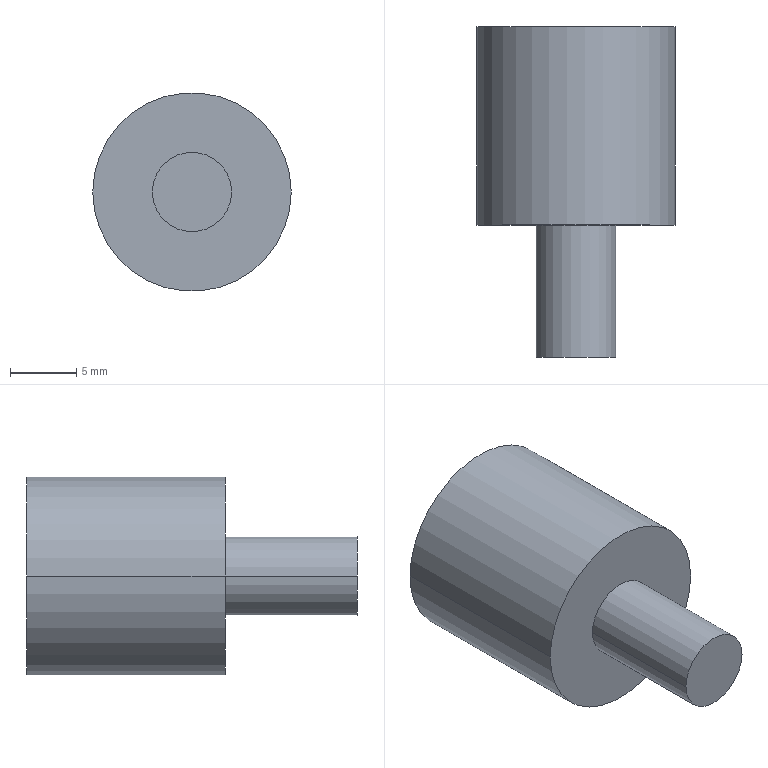Part | STEP file | SOLID | 1 solid | 15 faces | box 15 x 25 x 15 mm | volume 2709 mm3 | cylinder 8 | cone 4 | plane 3 | commonest cylinder face diameters 5 x2 6 x2 7.5 x2 15 x2
STEP:
#1=CARTESIAN_POINT('',(0.,0.,0.));
#2=DIRECTION('',(0.,0.,1.));
#3=DIRECTION('',(1.,0.,0.));
#4=AXIS2_PLACEMENT_3D('',#1,#2,#3);
#5=CARTESIAN_POINT('',(7.5,0.,0.));
#6=VERTEX_POINT('',#5);
#7=CARTESIAN_POINT('',(-7.5,0.,0.));
#8=VERTEX_POINT('',#7);
#9=CARTESIAN_POINT('',(0.,0.,0.));
#10=DIRECTION('',(0.,-1.,0.));
#11=DIRECTION('',(1.,0.,0.));
#12=AXIS2_PLACEMENT_3D('',#9,#10,#11);
#13=CIRCLE('',#12,7.5);
#14=CARTESIAN_POINT('',(0.,0.,0.));
#15=DIRECTION('',(0.,-1.,0.));
#16=DIRECTION('',(-1.,0.,0.));
#17=AXIS2_PLACEMENT_3D('',#14,#15,#16);
#18=PLANE('',#17);
#19=CARTESIAN_POINT('',(0.,0.));
#20=DIRECTION('',(-1.,0.));
#21=AXIS2_PLACEMENT_2D('',#19,#20);
#22=CIRCLE('',#21,7.5);
#23=(GEOMETRIC_REPRESENTATION_CONTEXT(2)PARAMETRIC_REPRESENTATION_CONTEXT()REPRESENTATION_CONTEXT('',''));
#24=DEFINITIONAL_REPRESENTATION('',(#22),#23);
#25=PCURVE('',#18,#24);
#26=CARTESIAN_POINT('',(0.,16.25,0.));
#27=DIRECTION('',(0.,-1.,0.));
#28=DIRECTION('',(-1.,0.,0.));
#29=AXIS2_PLACEMENT_3D('',#26,#27,#28);
#30=CYLINDRICAL_SURFACE('',#29,7.5);
#31=CARTESIAN_POINT('',(3.142,16.25));
#32=DIRECTION('',(1.,0.));
#33=VECTOR('',#32,1.);
#34=LINE('',#31,#33);
#35=(GEOMETRIC_REPRESENTATION_CONTEXT(2)PARAMETRIC_REPRESENTATION_CONTEXT()REPRESENTATION_CONTEXT('',''));
#36=DEFINITIONAL_REPRESENTATION('',(#34),#35);
#37=PCURVE('',#30,#36);
#38=SURFACE_CURVE('',#13,(#25,#37),.PCURVE_S1.);
#39=EDGE_CURVE('',#6,#8,#38,.T.);
#40=ORIENTED_EDGE('',*,*,#39,.F.);
#41=CARTESIAN_POINT('',(0.,0.,0.));
#42=DIRECTION('',(0.,1.,0.));
#43=DIRECTION('',(1.,0.,0.));
#44=AXIS2_PLACEMENT_3D('',#41,#42,#43);
#45=CIRCLE('',#44,7.5);
#46=CARTESIAN_POINT('',(-7.5,0.));
#47=CARTESIAN_POINT('',(-7.5,12.99));
#48=CARTESIAN_POINT('',(3.75,6.495));
#49=CARTESIAN_POINT('',(15.,0.));
#50=CARTESIAN_POINT('',(3.75,-6.495));
#51=CARTESIAN_POINT('',(-7.5,-12.99));
#52=CARTESIAN_POINT('',(-7.5,0.));
#53=(BOUNDED_CURVE()B_SPLINE_CURVE(2,(#46,#47,#48,#49,#50,#51,#52),.UNSPECIFIED.,.T.,.F.)B_SPLINE_CURVE_WITH_KNOTS((1,2,2,2,2,1),(-2.094,0.,2.094,4.189,6.283,8.378),.UNSPECIFIED.)CURVE()GEOMETRIC_REPRESENTATION_ITEM()RATIONAL_B_SPLINE_CURVE((1.,0.5,1.,0.5,1.,0.5,1.))REPRESENTATION_ITEM(''));
#54=(GEOMETRIC_REPRESENTATION_CONTEXT(2)PARAMETRIC_REPRESENTATION_CONTEXT()REPRESENTATION_CONTEXT('',''));
#55=DEFINITIONAL_REPRESENTATION('',(#53),#54);
#56=PCURVE('',#18,#55);
#57=CARTESIAN_POINT('',(0.,16.25,0.));
#58=DIRECTION('',(0.,-1.,0.));
#59=DIRECTION('',(-1.,0.,0.));
#60=AXIS2_PLACEMENT_3D('',#57,#58,#59);
#61=CYLINDRICAL_SURFACE('',#60,7.5);
#62=CARTESIAN_POINT('',(3.142,16.25));
#63=DIRECTION('',(-1.,0.));
#64=VECTOR('',#63,1.);
#65=LINE('',#62,#64);
#66=(GEOMETRIC_REPRESENTATION_CONTEXT(2)PARAMETRIC_REPRESENTATION_CONTEXT()REPRESENTATION_CONTEXT('',''));
#67=DEFINITIONAL_REPRESENTATION('',(#65),#66);
#68=PCURVE('',#61,#67);
#69=SURFACE_CURVE('',#45,(#56,#68),.PCURVE_S1.);
#70=EDGE_CURVE('',#6,#8,#69,.T.);
#71=ORIENTED_EDGE('',*,*,#70,.T.);
#72=EDGE_LOOP('',(#40,#71));
#73=FACE_BOUND('',#72,.F.);
#74=CARTESIAN_POINT('',(3.,0.,0.));
#75=VERTEX_POINT('',#74);
#76=CARTESIAN_POINT('',(-3.,0.,0.));
#77=VERTEX_POINT('',#76);
#78=CARTESIAN_POINT('',(0.,0.,0.));
#79=DIRECTION('',(0.,1.,0.));
#80=DIRECTION('',(1.,0.,0.));
#81=AXIS2_PLACEMENT_3D('',#78,#79,#80);
#82=CIRCLE('',#81,3.);
#83=CARTESIAN_POINT('',(-3.,0.));
#84=CARTESIAN_POINT('',(-3.,5.196));
#85=CARTESIAN_POINT('',(1.5,2.598));
#86=CARTESIAN_POINT('',(6.,0.));
#87=CARTESIAN_POINT('',(1.5,-2.598));
#88=CARTESIAN_POINT('',(-3.,-5.196));
#89=CARTESIAN_POINT('',(-3.,0.));
#90=(BOUNDED_CURVE()B_SPLINE_CURVE(2,(#83,#84,#85,#86,#87,#88,#89),.UNSPECIFIED.,.T.,.F.)B_SPLINE_CURVE_WITH_KNOTS((1,2,2,2,2,1),(-2.094,0.,2.094,4.189,6.283,8.378),.UNSPECIFIED.)CURVE()GEOMETRIC_REPRESENTATION_ITEM()RATIONAL_B_SPLINE_CURVE((1.,0.5,1.,0.5,1.,0.5,1.))REPRESENTATION_ITEM(''));
#91=(GEOMETRIC_REPRESENTATION_CONTEXT(2)PARAMETRIC_REPRESENTATION_CONTEXT()REPRESENTATION_CONTEXT('',''));
#92=DEFINITIONAL_REPRESENTATION('',(#90),#91);
#93=PCURVE('',#18,#92);
#94=CARTESIAN_POINT('',(0.,16.25,0.));
#95=DIRECTION('',(0.,-1.,0.));
#96=DIRECTION('',(-1.,0.,0.));
#97=AXIS2_PLACEMENT_3D('',#94,#95,#96);
#98=CYLINDRICAL_SURFACE('',#97,3.);
#99=CARTESIAN_POINT('',(3.142,16.25));
#100=DIRECTION('',(-1.,0.));
#101=VECTOR('',#100,1.);
#102=LINE('',#99,#101);
#103=(GEOMETRIC_REPRESENTATION_CONTEXT(2)PARAMETRIC_REPRESENTATION_CONTEXT()REPRESENTATION_CONTEXT('',''));
#104=DEFINITIONAL_REPRESENTATION('',(#102),#103);
#105=PCURVE('',#98,#104);
#106=SURFACE_CURVE('',#82,(#93,#105),.PCURVE_S1.);
#107=EDGE_CURVE('',#75,#77,#106,.T.);
#108=ORIENTED_EDGE('',*,*,#107,.F.);
#109=CARTESIAN_POINT('',(0.,0.,0.));
#110=DIRECTION('',(0.,-1.,0.));
#111=DIRECTION('',(1.,0.,0.));
#112=AXIS2_PLACEMENT_3D('',#109,#110,#111);
#113=CIRCLE('',#112,3.);
#114=CARTESIAN_POINT('',(0.,0.));
#115=DIRECTION('',(-1.,0.));
#116=AXIS2_PLACEMENT_2D('',#114,#115);
#117=CIRCLE('',#116,3.);
#118=(GEOMETRIC_REPRESENTATION_CONTEXT(2)PARAMETRIC_REPRESENTATION_CONTEXT()REPRESENTATION_CONTEXT('',''));
#119=DEFINITIONAL_REPRESENTATION('',(#117),#118);
#120=PCURVE('',#18,#119);
#121=CARTESIAN_POINT('',(0.,16.25,0.));
#122=DIRECTION('',(0.,-1.,0.));
#123=DIRECTION('',(-1.,0.,0.));
#124=AXIS2_PLACEMENT_3D('',#121,#122,#123);
#125=CYLINDRICAL_SURFACE('',#124,3.);
#126=CARTESIAN_POINT('',(3.142,16.25));
#127=DIRECTION('',(1.,0.));
#128=VECTOR('',#127,1.);
#129=LINE('',#126,#128);
#130=(GEOMETRIC_REPRESENTATION_CONTEXT(2)PARAMETRIC_REPRESENTATION_CONTEXT()REPRESENTATION_CONTEXT('',''));
#131=DEFINITIONAL_REPRESENTATION('',(#129),#130);
#132=PCURVE('',#125,#131);
#133=SURFACE_CURVE('',#113,(#120,#132),.PCURVE_S1.);
#134=EDGE_CURVE('',#75,#77,#133,.T.);
#135=ORIENTED_EDGE('',*,*,#134,.T.);
#136=EDGE_LOOP('',(#108,#135));
#137=FACE_BOUND('',#136,.F.);
#138=ADVANCED_FACE('',(#73,#137),#18,.T.);
#139=CARTESIAN_POINT('',(7.5,15.,0.));
#140=VERTEX_POINT('',#139);
#141=CARTESIAN_POINT('',(-7.5,15.,0.));
#142=VERTEX_POINT('',#141);
#143=CARTESIAN_POINT('',(0.,15.,0.));
#144=DIRECTION('',(0.,-1.,0.));
#145=DIRECTION('',(1.,0.,0.));
#146=AXIS2_PLACEMENT_3D('',#143,#144,#145);
#147=CIRCLE('',#146,7.5);
#148=CARTESIAN_POINT('',(3.142,1.25));
#149=DIRECTION('',(1.,0.));
#150=VECTOR('',#149,1.);
#151=LINE('',#148,#150);
#152=(GEOMETRIC_REPRESENTATION_CONTEXT(2)PARAMETRIC_REPRESENTATION_CONTEXT()REPRESENTATION_CONTEXT('',''));
#153=DEFINITIONAL_REPRESENTATION('',(#151),#152);
#154=PCURVE('',#30,#153);
#155=CARTESIAN_POINT('',(0.,15.,0.));
#156=DIRECTION('',(0.,-1.,0.));
#157=DIRECTION('',(-1.,0.,0.));
#158=AXIS2_PLACEMENT_3D('',#155,#156,#157);
#159=PLANE('',#158);
#160=CARTESIAN_POINT('',(0.,0.));
#161=DIRECTION('',(-1.,0.));
#162=AXIS2_PLACEMENT_2D('',#160,#161);
#163=CIRCLE('',#162,7.5);
#164=(GEOMETRIC_REPRESENTATION_CONTEXT(2)PARAMETRIC_REPRESENTATION_CONTEXT()REPRESENTATION_CONTEXT('',''));
#165=DEFINITIONAL_REPRESENTATION('',(#163),#164);
#166=PCURVE('',#159,#165);
#167=SURFACE_CURVE('',#147,(#154,#166),.PCURVE_S1.);
#168=EDGE_CURVE('',#140,#142,#167,.T.);
#169=ORIENTED_EDGE('',*,*,#168,.T.);
#170=CARTESIAN_POINT('',(-7.5,0.,0.));
#171=DIRECTION('',(0.,1.,0.));
#172=VECTOR('',#171,1.);
#173=LINE('',#170,#172);
#174=CARTESIAN_POINT('',(6.283,16.25));
#175=DIRECTION('',(0.,-1.));
#176=VECTOR('',#175,1.);
#177=LINE('',#174,#176);
#178=(GEOMETRIC_REPRESENTATION_CONTEXT(2)PARAMETRIC_REPRESENTATION_CONTEXT()REPRESENTATION_CONTEXT('',''));
#179=DEFINITIONAL_REPRESENTATION('',(#177),#178);
#180=PCURVE('',#30,#179);
#181=CARTESIAN_POINT('',(0.,16.25));
#182=DIRECTION('',(0.,-1.));
#183=VECTOR('',#182,1.);
#184=LINE('',#181,#183);
#185=(GEOMETRIC_REPRESENTATION_CONTEXT(2)PARAMETRIC_REPRESENTATION_CONTEXT()REPRESENTATION_CONTEXT('',''));
#186=DEFINITIONAL_REPRESENTATION('',(#184),#185);
#187=PCURVE('',#61,#186);
#188=SURFACE_CURVE('',#173,(#180,#187),.PCURVE_S1.);
#189=EDGE_CURVE('',#8,#142,#188,.T.);
#190=ORIENTED_EDGE('',*,*,#189,.F.);
#191=ORIENTED_EDGE('',*,*,#39,.F.);
#192=CARTESIAN_POINT('',(7.5,0.,0.));
#193=DIRECTION('',(0.,1.,0.));
#194=VECTOR('',#193,1.);
#195=LINE('',#192,#194);
#196=CARTESIAN_POINT('',(3.142,16.25));
#197=DIRECTION('',(0.,-1.));
#198=VECTOR('',#197,1.);
#199=LINE('',#196,#198);
#200=(GEOMETRIC_REPRESENTATION_CONTEXT(2)PARAMETRIC_REPRESENTATION_CONTEXT()REPRESENTATION_CONTEXT('',''));
#201=DEFINITIONAL_REPRESENTATION('',(#199),#200);
#202=PCURVE('',#30,#201);
#203=CARTESIAN_POINT('',(3.142,16.25));
#204=DIRECTION('',(0.,-1.));
#205=VECTOR('',#204,1.);
#206=LINE('',#203,#205);
#207=(GEOMETRIC_REPRESENTATION_CONTEXT(2)PARAMETRIC_REPRESENTATION_CONTEXT()REPRESENTATION_CONTEXT('',''));
#208=DEFINITIONAL_REPRESENTATION('',(#206),#207);
#209=PCURVE('',#61,#208);
#210=SURFACE_CURVE('',#195,(#202,#209),.PCURVE_S1.);
#211=EDGE_CURVE('',#6,#140,#210,.T.);
#212=ORIENTED_EDGE('',*,*,#211,.T.);
#213=EDGE_LOOP('',(#169,#190,#191,#212));
#214=FACE_BOUND('',#213,.T.);
#215=ADVANCED_FACE('',(#214),#30,.T.);
#216=ORIENTED_EDGE('',*,*,#70,.T.);
#217=ORIENTED_EDGE('',*,*,#189,.T.);
#218=CARTESIAN_POINT('',(0.,15.,0.));
#219=DIRECTION('',(0.,1.,0.));
#220=DIRECTION('',(1.,0.,0.));
#221=AXIS2_PLACEMENT_3D('',#218,#219,#220);
#222=CIRCLE('',#221,7.5);
#223=CARTESIAN_POINT('',(3.142,1.25));
#224=DIRECTION('',(-1.,0.));
#225=VECTOR('',#224,1.);
#226=LINE('',#223,#225);
#227=(GEOMETRIC_REPRESENTATION_CONTEXT(2)PARAMETRIC_REPRESENTATION_CONTEXT()REPRESENTATION_CONTEXT('',''));
#228=DEFINITIONAL_REPRESENTATION('',(#226),#227);
#229=PCURVE('',#61,#228);
#230=CARTESIAN_POINT('',(-7.5,0.));
#231=CARTESIAN_POINT('',(-7.5,12.99));
#232=CARTESIAN_POINT('',(3.75,6.495));
#233=CARTESIAN_POINT('',(15.,0.));
#234=CARTESIAN_POINT('',(3.75,-6.495));
#235=CARTESIAN_POINT('',(-7.5,-12.99));
#236=CARTESIAN_POINT('',(-7.5,0.));
#237=(BOUNDED_CURVE()B_SPLINE_CURVE(2,(#230,#231,#232,#233,#234,#235,#236),.UNSPECIFIED.,.T.,.F.)B_SPLINE_CURVE_WITH_KNOTS((1,2,2,2,2,1),(-2.094,0.,2.094,4.189,6.283,8.378),.UNSPECIFIED.)CURVE()GEOMETRIC_REPRESENTATION_ITEM()RATIONAL_B_SPLINE_CURVE((1.,0.5,1.,0.5,1.,0.5,1.))REPRESENTATION_ITEM(''));
#238=(GEOMETRIC_REPRESENTATION_CONTEXT(2)PARAMETRIC_REPRESENTATION_CONTEXT()REPRESENTATION_CONTEXT('',''));
#239=DEFINITIONAL_REPRESENTATION('',(#237),#238);
#240=PCURVE('',#159,#239);
#241=SURFACE_CURVE('',#222,(#229,#240),.PCURVE_S1.);
#242=EDGE_CURVE('',#140,#142,#241,.T.);
#243=ORIENTED_EDGE('',*,*,#242,.F.);
#244=ORIENTED_EDGE('',*,*,#211,.F.);
#245=EDGE_LOOP('',(#216,#217,#243,#244));
#246=FACE_BOUND('',#245,.T.);
#247=ADVANCED_FACE('',(#246),#61,.T.);
#248=ORIENTED_EDGE('',*,*,#242,.F.);
#249=ORIENTED_EDGE('',*,*,#168,.T.);
#250=EDGE_LOOP('',(#248,#249));
#251=FACE_BOUND('',#250,.F.);
#252=CARTESIAN_POINT('',(-3.75,15.,0.));
#253=VERTEX_POINT('',#252);
#254=CARTESIAN_POINT('',(3.75,15.,0.));
#255=VERTEX_POINT('',#254);
#256=CARTESIAN_POINT('',(0.,15.,0.));
#257=DIRECTION('',(0.,-1.,0.));
#258=DIRECTION('',(-1.,0.,0.));
#259=AXIS2_PLACEMENT_3D('',#256,#257,#258);
#260=CIRCLE('',#259,3.75);
#261=CARTESIAN_POINT('',(0.,0.));
#262=DIRECTION('',(1.,0.));
#263=AXIS2_PLACEMENT_2D('',#261,#262);
#264=CIRCLE('',#263,3.75);
#265=(GEOMETRIC_REPRESENTATION_CONTEXT(2)PARAMETRIC_REPRESENTATION_CONTEXT()REPRESENTATION_CONTEXT('',''));
#266=DEFINITIONAL_REPRESENTATION('',(#264),#265);
#267=PCURVE('',#159,#266);
#268=CARTESIAN_POINT('',(0.,15.213,0.));
#269=DIRECTION('',(0.,-1.,0.));
#270=DIRECTION('',(-1.,0.,0.));
#271=AXIS2_PLACEMENT_3D('',#268,#269,#270);
#272=CYLINDRICAL_SURFACE('',#271,3.75);
#273=CARTESIAN_POINT('',(0.,0.2127));
#274=DIRECTION('',(1.,0.));
#275=VECTOR('',#274,1.);
#276=LINE('',#273,#275);
#277=(GEOMETRIC_REPRESENTATION_CONTEXT(2)PARAMETRIC_REPRESENTATION_CONTEXT()REPRESENTATION_CONTEXT('',''));
#278=DEFINITIONAL_REPRESENTATION('',(#276),#277);
#279=PCURVE('',#272,#278);
#280=SURFACE_CURVE('',#260,(#267,#279),.PCURVE_S1.);
#281=EDGE_CURVE('',#253,#255,#280,.T.);
#282=ORIENTED_EDGE('',*,*,#281,.F.);
#283=CARTESIAN_POINT('',(0.,15.,0.));
#284=DIRECTION('',(0.,-1.,0.));
#285=DIRECTION('',(1.,0.,0.));
#286=AXIS2_PLACEMENT_3D('',#283,#284,#285);
#287=CIRCLE('',#286,3.75);
#288=CARTESIAN_POINT('',(0.,0.));
#289=DIRECTION('',(-1.,0.));
#290=AXIS2_PLACEMENT_2D('',#288,#289);
#291=CIRCLE('',#290,3.75);
#292=(GEOMETRIC_REPRESENTATION_CONTEXT(2)PARAMETRIC_REPRESENTATION_CONTEXT()REPRESENTATION_CONTEXT('',''));
#293=DEFINITIONAL_REPRESENTATION('',(#291),#292);
#294=PCURVE('',#159,#293);
#295=CARTESIAN_POINT('',(0.,15.213,0.));
#296=DIRECTION('',(0.,-1.,0.));
#297=DIRECTION('',(-1.,0.,0.));
#298=AXIS2_PLACEMENT_3D('',#295,#296,#297);
#299=CYLINDRICAL_SURFACE('',#298,3.75);
#300=CARTESIAN_POINT('',(3.142,0.2127));
#301=DIRECTION('',(1.,0.));
#302=VECTOR('',#301,1.);
#303=LINE('',#300,#302);
#304=(GEOMETRIC_REPRESENTATION_CONTEXT(2)PARAMETRIC_REPRESENTATION_CONTEXT()REPRESENTATION_CONTEXT('',''));
#305=DEFINITIONAL_REPRESENTATION('',(#303),#304);
#306=PCURVE('',#299,#305);
#307=SURFACE_CURVE('',#287,(#294,#306),.PCURVE_S1.);
#308=EDGE_CURVE('',#255,#253,#307,.T.);
#309=ORIENTED_EDGE('',*,*,#308,.F.);
#310=EDGE_LOOP('',(#282,#309));
#311=FACE_BOUND('',#310,.F.);
#312=ADVANCED_FACE('',(#251,#311),#159,.F.);
#313=ORIENTED_EDGE('',*,*,#281,.T.);
#314=CARTESIAN_POINT('',(3.75,13.,0.));
#315=VERTEX_POINT('',#314);
#316=CARTESIAN_POINT('',(3.75,15.,0.));
#317=DIRECTION('',(0.,-1.,0.));
#318=VECTOR('',#317,1.);
#319=LINE('',#316,#318);
#320=CARTESIAN_POINT('',(3.142,0.2127));
#321=DIRECTION('',(0.,1.));
#322=VECTOR('',#321,1.);
#323=LINE('',#320,#322);
#324=(GEOMETRIC_REPRESENTATION_CONTEXT(2)PARAMETRIC_REPRESENTATION_CONTEXT()REPRESENTATION_CONTEXT('',''));
#325=DEFINITIONAL_REPRESENTATION('',(#323),#324);
#326=PCURVE('',#272,#325);
#327=CARTESIAN_POINT('',(3.142,0.2127));
#328=DIRECTION('',(0.,1.));
#329=VECTOR('',#328,1.);
#330=LINE('',#327,#329);
#331=(GEOMETRIC_REPRESENTATION_CONTEXT(2)PARAMETRIC_REPRESENTATION_CONTEXT()REPRESENTATION_CONTEXT('',''));
#332=DEFINITIONAL_REPRESENTATION('',(#330),#331);
#333=PCURVE('',#299,#332);
#334=SURFACE_CURVE('',#319,(#326,#333),.PCURVE_S1.);
#335=EDGE_CURVE('',#255,#315,#334,.T.);
#336=ORIENTED_EDGE('',*,*,#335,.T.);
#337=CARTESIAN_POINT('',(-3.75,13.,0.));
#338=VERTEX_POINT('',#337);
#339=CARTESIAN_POINT('',(0.,13.,0.));
#340=DIRECTION('',(0.,-1.,0.));
#341=DIRECTION('',(-1.,0.,0.));
#342=AXIS2_PLACEMENT_3D('',#339,#340,#341);
#343=CIRCLE('',#342,3.75);
#344=CARTESIAN_POINT('',(0.,2.213));
#345=DIRECTION('',(1.,0.));
#346=VECTOR('',#345,1.);
#347=LINE('',#344,#346);
#348=(GEOMETRIC_REPRESENTATION_CONTEXT(2)PARAMETRIC_REPRESENTATION_CONTEXT()REPRESENTATION_CONTEXT('',''));
#349=DEFINITIONAL_REPRESENTATION('',(#347),#348);
#350=PCURVE('',#272,#349);
#351=CARTESIAN_POINT('',(0.,12.624,0.));
#352=DIRECTION('',(0.,1.,0.));
#353=DIRECTION('',(1.,0.,0.));
#354=AXIS2_PLACEMENT_3D('',#351,#352,#353);
#355=CONICAL_SURFACE('',#354,3.125,1.03);
#356=CARTESIAN_POINT('',(3.142,0.3755));
#357=DIRECTION('',(-1.,0.));
#358=VECTOR('',#357,1.);
#359=LINE('',#356,#358);
#360=(GEOMETRIC_REPRESENTATION_CONTEXT(2)PARAMETRIC_REPRESENTATION_CONTEXT()REPRESENTATION_CONTEXT('',''));
#361=DEFINITIONAL_REPRESENTATION('',(#359),#360);
#362=PCURVE('',#355,#361);
#363=SURFACE_CURVE('',#343,(#350,#362),.PCURVE_S1.);
#364=EDGE_CURVE('',#338,#315,#363,.T.);
#365=ORIENTED_EDGE('',*,*,#364,.F.);
#366=CARTESIAN_POINT('',(-3.75,15.,0.));
#367=DIRECTION('',(0.,-1.,0.));
#368=VECTOR('',#367,1.);
#369=LINE('',#366,#368);
#370=CARTESIAN_POINT('',(0.,0.2127));
#371=DIRECTION('',(0.,1.));
#372=VECTOR('',#371,1.);
#373=LINE('',#370,#372);
#374=(GEOMETRIC_REPRESENTATION_CONTEXT(2)PARAMETRIC_REPRESENTATION_CONTEXT()REPRESENTATION_CONTEXT('',''));
#375=DEFINITIONAL_REPRESENTATION('',(#373),#374);
#376=PCURVE('',#272,#375);
#377=CARTESIAN_POINT('',(6.283,0.2127));
#378=DIRECTION('',(0.,1.));
#379=VECTOR('',#378,1.);
#380=LINE('',#377,#379);
#381=(GEOMETRIC_REPRESENTATION_CONTEXT(2)PARAMETRIC_REPRESENTATION_CONTEXT()REPRESENTATION_CONTEXT('',''));
#382=DEFINITIONAL_REPRESENTATION('',(#380),#381);
#383=PCURVE('',#299,#382);
#384=SURFACE_CURVE('',#369,(#376,#383),.PCURVE_S1.);
#385=EDGE_CURVE('',#253,#338,#384,.T.);
#386=ORIENTED_EDGE('',*,*,#385,.F.);
#387=EDGE_LOOP('',(#313,#336,#365,#386));
#388=FACE_BOUND('',#387,.F.);
#389=ADVANCED_FACE('',(#388),#272,.F.);
#390=ORIENTED_EDGE('',*,*,#308,.T.);
#391=ORIENTED_EDGE('',*,*,#385,.T.);
#392=CARTESIAN_POINT('',(0.,13.,0.));
#393=DIRECTION('',(0.,1.,0.));
#394=DIRECTION('',(-1.,0.,0.));
#395=AXIS2_PLACEMENT_3D('',#392,#393,#394);
#396=CIRCLE('',#395,3.75);
#397=CARTESIAN_POINT('',(6.283,2.213));
#398=DIRECTION('',(-1.,0.));
#399=VECTOR('',#398,1.);
#400=LINE('',#397,#399);
#401=(GEOMETRIC_REPRESENTATION_CONTEXT(2)PARAMETRIC_REPRESENTATION_CONTEXT()REPRESENTATION_CONTEXT('',''));
#402=DEFINITIONAL_REPRESENTATION('',(#400),#401);
#403=PCURVE('',#299,#402);
#404=CARTESIAN_POINT('',(0.,12.624,0.));
#405=DIRECTION('',(0.,1.,0.));
#406=DIRECTION('',(1.,0.,0.));
#407=AXIS2_PLACEMENT_3D('',#404,#405,#406);
#408=CONICAL_SURFACE('',#407,3.125,1.03);
#409=CARTESIAN_POINT('',(3.142,0.3755));
#410=DIRECTION('',(1.,0.));
#411=VECTOR('',#410,1.);
#412=LINE('',#409,#411);
#413=(GEOMETRIC_REPRESENTATION_CONTEXT(2)PARAMETRIC_REPRESENTATION_CONTEXT()REPRESENTATION_CONTEXT('',''));
#414=DEFINITIONAL_REPRESENTATION('',(#412),#413);
#415=PCURVE('',#408,#414);
#416=SURFACE_CURVE('',#396,(#403,#415),.PCURVE_S1.);
#417=EDGE_CURVE('',#338,#315,#416,.T.);
#418=ORIENTED_EDGE('',*,*,#417,.T.);
#419=ORIENTED_EDGE('',*,*,#335,.F.);
#420=EDGE_LOOP('',(#390,#391,#418,#419));
#421=FACE_BOUND('',#420,.F.);
#422=ADVANCED_FACE('',(#421),#299,.F.);
#423=CARTESIAN_POINT('',(-2.5,12.249,0.));
#424=VERTEX_POINT('',#423);
#425=CARTESIAN_POINT('',(2.5,12.249,0.));
#426=VERTEX_POINT('',#425);
#427=CARTESIAN_POINT('',(0.,12.249,0.));
#428=DIRECTION('',(0.,1.,0.));
#429=DIRECTION('',(-1.,0.,0.));
#430=AXIS2_PLACEMENT_3D('',#427,#428,#429);
#431=CIRCLE('',#430,2.5);
#432=CARTESIAN_POINT('',(3.142,-0.3755));
#433=DIRECTION('',(1.,0.));
#434=VECTOR('',#433,1.);
#435=LINE('',#432,#434);
#436=(GEOMETRIC_REPRESENTATION_CONTEXT(2)PARAMETRIC_REPRESENTATION_CONTEXT()REPRESENTATION_CONTEXT('',''));
#437=DEFINITIONAL_REPRESENTATION('',(#435),#436);
#438=PCURVE('',#408,#437);
#439=CARTESIAN_POINT('',(0.,5.023,0.));
#440=DIRECTION('',(0.,1.,0.));
#441=DIRECTION('',(1.,0.,0.));
#442=AXIS2_PLACEMENT_3D('',#439,#440,#441);
#443=CYLINDRICAL_SURFACE('',#442,2.5);
#444=CARTESIAN_POINT('',(3.142,7.226));
#445=DIRECTION('',(1.,0.));
#446=VECTOR('',#445,1.);
#447=LINE('',#444,#446);
#448=(GEOMETRIC_REPRESENTATION_CONTEXT(2)PARAMETRIC_REPRESENTATION_CONTEXT()REPRESENTATION_CONTEXT('',''));
#449=DEFINITIONAL_REPRESENTATION('',(#447),#448);
#450=PCURVE('',#443,#449);
#451=SURFACE_CURVE('',#431,(#438,#450),.PCURVE_S1.);
#452=EDGE_CURVE('',#424,#426,#451,.T.);
#453=ORIENTED_EDGE('',*,*,#452,.T.);
#454=CARTESIAN_POINT('',(3.75,13.,0.));
#455=DIRECTION('',(-0.8572,-0.515,0.));
#456=VECTOR('',#455,1.);
#457=LINE('',#454,#456);
#458=CARTESIAN_POINT('',(6.283,0.3755));
#459=DIRECTION('',(0.,-1.));
#460=VECTOR('',#459,1.);
#461=LINE('',#458,#460);
#462=(GEOMETRIC_REPRESENTATION_CONTEXT(2)PARAMETRIC_REPRESENTATION_CONTEXT()REPRESENTATION_CONTEXT('',''));
#463=DEFINITIONAL_REPRESENTATION('',(#461),#462);
#464=PCURVE('',#408,#463);
#465=CARTESIAN_POINT('',(0.,0.3755));
#466=DIRECTION('',(0.,-1.));
#467=VECTOR('',#466,1.);
#468=LINE('',#465,#467);
#469=(GEOMETRIC_REPRESENTATION_CONTEXT(2)PARAMETRIC_REPRESENTATION_CONTEXT()REPRESENTATION_CONTEXT('',''));
#470=DEFINITIONAL_REPRESENTATION('',(#468),#469);
#471=PCURVE('',#355,#470);
#472=SURFACE_CURVE('',#457,(#464,#471),.PCURVE_S1.);
#473=EDGE_CURVE('',#315,#426,#472,.T.);
#474=ORIENTED_EDGE('',*,*,#473,.F.);
#475=ORIENTED_EDGE('',*,*,#417,.F.);
#476=CARTESIAN_POINT('',(-3.75,13.,0.));
#477=DIRECTION('',(0.8572,-0.515,0.));
#478=VECTOR('',#477,1.);
#479=LINE('',#476,#478);
#480=CARTESIAN_POINT('',(3.142,0.3755));
#481=DIRECTION('',(0.,-1.));
#482=VECTOR('',#481,1.);
#483=LINE('',#480,#482);
#484=(GEOMETRIC_REPRESENTATION_CONTEXT(2)PARAMETRIC_REPRESENTATION_CONTEXT()REPRESENTATION_CONTEXT('',''));
#485=DEFINITIONAL_REPRESENTATION('',(#483),#484);
#486=PCURVE('',#408,#485);
#487=CARTESIAN_POINT('',(3.142,0.3755));
#488=DIRECTION('',(0.,-1.));
#489=VECTOR('',#488,1.);
#490=LINE('',#487,#489);
#491=(GEOMETRIC_REPRESENTATION_CONTEXT(2)PARAMETRIC_REPRESENTATION_CONTEXT()REPRESENTATION_CONTEXT('',''));
#492=DEFINITIONAL_REPRESENTATION('',(#490),#491);
#493=PCURVE('',#355,#492);
#494=SURFACE_CURVE('',#479,(#486,#493),.PCURVE_S1.);
#495=EDGE_CURVE('',#338,#424,#494,.T.);
#496=ORIENTED_EDGE('',*,*,#495,.T.);
#497=EDGE_LOOP('',(#453,#474,#475,#496));
#498=FACE_BOUND('',#497,.F.);
#499=ADVANCED_FACE('',(#498),#408,.F.);
#500=ORIENTED_EDGE('',*,*,#452,.F.);
#501=CARTESIAN_POINT('',(-2.5,7.,0.));
#502=VERTEX_POINT('',#501);
#503=CARTESIAN_POINT('',(-2.5,7.,0.));
#504=DIRECTION('',(0.,1.,0.));
#505=VECTOR('',#504,1.);
#506=LINE('',#503,#505);
#507=CARTESIAN_POINT('',(3.142,1.977));
#508=DIRECTION('',(0.,1.));
#509=VECTOR('',#508,1.);
#510=LINE('',#507,#509);
#511=(GEOMETRIC_REPRESENTATION_CONTEXT(2)PARAMETRIC_REPRESENTATION_CONTEXT()REPRESENTATION_CONTEXT('',''));
#512=DEFINITIONAL_REPRESENTATION('',(#510),#511);
#513=PCURVE('',#443,#512);
#514=CARTESIAN_POINT('',(0.,5.023,0.));
#515=DIRECTION('',(0.,1.,0.));
#516=DIRECTION('',(1.,0.,0.));
#517=AXIS2_PLACEMENT_3D('',#514,#515,#516);
#518=CYLINDRICAL_SURFACE('',#517,2.5);
#519=CARTESIAN_POINT('',(3.142,1.977));
#520=DIRECTION('',(0.,1.));
#521=VECTOR('',#520,1.);
#522=LINE('',#519,#521);
#523=(GEOMETRIC_REPRESENTATION_CONTEXT(2)PARAMETRIC_REPRESENTATION_CONTEXT()REPRESENTATION_CONTEXT('',''));
#524=DEFINITIONAL_REPRESENTATION('',(#522),#523);
#525=PCURVE('',#518,#524);
#526=SURFACE_CURVE('',#506,(#513,#525),.PCURVE_S1.);
#527=EDGE_CURVE('',#502,#424,#526,.T.);
#528=ORIENTED_EDGE('',*,*,#527,.F.);
#529=CARTESIAN_POINT('',(2.5,7.,0.));
#530=VERTEX_POINT('',#529);
#531=CARTESIAN_POINT('',(0.,7.,0.));
#532=DIRECTION('',(0.,-1.,0.));
#533=DIRECTION('',(1.,0.,0.));
#534=AXIS2_PLACEMENT_3D('',#531,#532,#533);
#535=CIRCLE('',#534,2.5);
#536=CARTESIAN_POINT('',(6.283,1.977));
#537=DIRECTION('',(-1.,0.));
#538=VECTOR('',#537,1.);
#539=LINE('',#536,#538);
#540=(GEOMETRIC_REPRESENTATION_CONTEXT(2)PARAMETRIC_REPRESENTATION_CONTEXT()REPRESENTATION_CONTEXT('',''));
#541=DEFINITIONAL_REPRESENTATION('',(#539),#540);
#542=PCURVE('',#443,#541);
#543=CARTESIAN_POINT('',(0.,6.264,0.));
#544=DIRECTION('',(0.,1.,0.));
#545=DIRECTION('',(1.,0.,0.));
#546=AXIS2_PLACEMENT_3D('',#543,#544,#545);
#547=CONICAL_SURFACE('',#546,1.275,1.03);
#548=CARTESIAN_POINT('',(6.283,0.7361));
#549=DIRECTION('',(-1.,0.));
#550=VECTOR('',#549,1.);
#551=LINE('',#548,#550);
#552=(GEOMETRIC_REPRESENTATION_CONTEXT(2)PARAMETRIC_REPRESENTATION_CONTEXT()REPRESENTATION_CONTEXT('',''));
#553=DEFINITIONAL_REPRESENTATION('',(#551),#552);
#554=PCURVE('',#547,#553);
#555=SURFACE_CURVE('',#535,(#542,#554),.PCURVE_S1.);
#556=EDGE_CURVE('',#530,#502,#555,.T.);
#557=ORIENTED_EDGE('',*,*,#556,.F.);
#558=CARTESIAN_POINT('',(2.5,7.,0.));
#559=DIRECTION('',(0.,1.,0.));
#560=VECTOR('',#559,1.);
#561=LINE('',#558,#560);
#562=CARTESIAN_POINT('',(6.283,1.977));
#563=DIRECTION('',(0.,1.));
#564=VECTOR('',#563,1.);
#565=LINE('',#562,#564);
#566=(GEOMETRIC_REPRESENTATION_CONTEXT(2)PARAMETRIC_REPRESENTATION_CONTEXT()REPRESENTATION_CONTEXT('',''));
#567=DEFINITIONAL_REPRESENTATION('',(#565),#566);
#568=PCURVE('',#443,#567);
#569=CARTESIAN_POINT('',(0.,1.977));
#570=DIRECTION('',(0.,1.));
#571=VECTOR('',#570,1.);
#572=LINE('',#569,#571);
#573=(GEOMETRIC_REPRESENTATION_CONTEXT(2)PARAMETRIC_REPRESENTATION_CONTEXT()REPRESENTATION_CONTEXT('',''));
#574=DEFINITIONAL_REPRESENTATION('',(#572),#573);
#575=PCURVE('',#518,#574);
#576=SURFACE_CURVE('',#561,(#568,#575),.PCURVE_S1.);
#577=EDGE_CURVE('',#530,#426,#576,.T.);
#578=ORIENTED_EDGE('',*,*,#577,.T.);
#579=EDGE_LOOP('',(#500,#528,#557,#578));
#580=FACE_BOUND('',#579,.F.);
#581=ADVANCED_FACE('',(#580),#443,.F.);
#582=CARTESIAN_POINT('',(0.,12.249,0.));
#583=DIRECTION('',(0.,1.,0.));
#584=DIRECTION('',(1.,0.,0.));
#585=AXIS2_PLACEMENT_3D('',#582,#583,#584);
#586=CIRCLE('',#585,2.5);
#587=CARTESIAN_POINT('',(0.,7.226));
#588=DIRECTION('',(1.,0.));
#589=VECTOR('',#588,1.);
#590=LINE('',#587,#589);
#591=(GEOMETRIC_REPRESENTATION_CONTEXT(2)PARAMETRIC_REPRESENTATION_CONTEXT()REPRESENTATION_CONTEXT('',''));
#592=DEFINITIONAL_REPRESENTATION('',(#590),#591);
#593=PCURVE('',#518,#592);
#594=CARTESIAN_POINT('',(0.,-0.3755));
#595=DIRECTION('',(1.,0.));
#596=VECTOR('',#595,1.);
#597=LINE('',#594,#596);
#598=(GEOMETRIC_REPRESENTATION_CONTEXT(2)PARAMETRIC_REPRESENTATION_CONTEXT()REPRESENTATION_CONTEXT('',''));
#599=DEFINITIONAL_REPRESENTATION('',(#597),#598);
#600=PCURVE('',#355,#599);
#601=SURFACE_CURVE('',#586,(#593,#600),.PCURVE_S1.);
#602=EDGE_CURVE('',#426,#424,#601,.T.);
#603=ORIENTED_EDGE('',*,*,#602,.F.);
#604=ORIENTED_EDGE('',*,*,#577,.F.);
#605=CARTESIAN_POINT('',(0.,7.,0.));
#606=DIRECTION('',(0.,1.,0.));
#607=DIRECTION('',(1.,0.,0.));
#608=AXIS2_PLACEMENT_3D('',#605,#606,#607);
#609=CIRCLE('',#608,2.5);
#610=CARTESIAN_POINT('',(0.,1.977));
#611=DIRECTION('',(1.,0.));
#612=VECTOR('',#611,1.);
#613=LINE('',#610,#612);
#614=(GEOMETRIC_REPRESENTATION_CONTEXT(2)PARAMETRIC_REPRESENTATION_CONTEXT()REPRESENTATION_CONTEXT('',''));
#615=DEFINITIONAL_REPRESENTATION('',(#613),#614);
#616=PCURVE('',#518,#615);
#617=CARTESIAN_POINT('',(0.,6.264,0.));
#618=DIRECTION('',(0.,1.,0.));
#619=DIRECTION('',(1.,0.,0.));
#620=AXIS2_PLACEMENT_3D('',#617,#618,#619);
#621=CONICAL_SURFACE('',#620,1.275,1.03);
#622=CARTESIAN_POINT('',(0.,0.7361));
#623=DIRECTION('',(1.,0.));
#624=VECTOR('',#623,1.);
#625=LINE('',#622,#624);
#626=(GEOMETRIC_REPRESENTATION_CONTEXT(2)PARAMETRIC_REPRESENTATION_CONTEXT()REPRESENTATION_CONTEXT('',''));
#627=DEFINITIONAL_REPRESENTATION('',(#625),#626);
#628=PCURVE('',#621,#627);
#629=SURFACE_CURVE('',#609,(#616,#628),.PCURVE_S1.);
#630=EDGE_CURVE('',#530,#502,#629,.T.);
#631=ORIENTED_EDGE('',*,*,#630,.T.);
#632=ORIENTED_EDGE('',*,*,#527,.T.);
#633=EDGE_LOOP('',(#603,#604,#631,#632));
#634=FACE_BOUND('',#633,.F.);
#635=ADVANCED_FACE('',(#634),#518,.F.);
#636=ORIENTED_EDGE('',*,*,#602,.T.);
#637=ORIENTED_EDGE('',*,*,#495,.F.);
#638=ORIENTED_EDGE('',*,*,#364,.T.);
#639=ORIENTED_EDGE('',*,*,#473,.T.);
#640=EDGE_LOOP('',(#636,#637,#638,#639));
#641=FACE_BOUND('',#640,.F.);
#642=ADVANCED_FACE('',(#641),#355,.F.);
#643=CARTESIAN_POINT('',(0.,5.498,0.));
#644=VERTEX_POINT('',#643);
#645=CARTESIAN_POINT('',(0.,5.498,0.));
#646=DIRECTION('',(0.8572,0.515,0.));
#647=VECTOR('',#646,1.);
#648=LINE('',#645,#647);
#649=CARTESIAN_POINT('',(0.,-0.7661));
#650=DIRECTION('',(0.,1.));
#651=VECTOR('',#650,1.);
#652=LINE('',#649,#651);
#653=(GEOMETRIC_REPRESENTATION_CONTEXT(2)PARAMETRIC_REPRESENTATION_CONTEXT()REPRESENTATION_CONTEXT('',''));
#654=DEFINITIONAL_REPRESENTATION('',(#652),#653);
#655=PCURVE('',#621,#654);
#656=CARTESIAN_POINT('',(6.283,-0.7661));
#657=DIRECTION('',(0.,1.));
#658=VECTOR('',#657,1.);
#659=LINE('',#656,#658);
#660=(GEOMETRIC_REPRESENTATION_CONTEXT(2)PARAMETRIC_REPRESENTATION_CONTEXT()REPRESENTATION_CONTEXT('',''));
#661=DEFINITIONAL_REPRESENTATION('',(#659),#660);
#662=PCURVE('',#547,#661);
#663=SURFACE_CURVE('',#648,(#655,#662),.PCURVE_S1.);
#664=EDGE_CURVE('',#644,#530,#663,.T.);
#665=ORIENTED_EDGE('',*,*,#664,.F.);
#666=CARTESIAN_POINT('',(0.,5.498,0.));
#667=DIRECTION('',(-0.8572,0.515,0.));
#668=VECTOR('',#667,1.);
#669=LINE('',#666,#668);
#670=CARTESIAN_POINT('',(3.142,-0.7661));
#671=CARTESIAN_POINT('',(3.142,-0.7433));
#672=CARTESIAN_POINT('',(3.142,-0.6978));
#673=CARTESIAN_POINT('',(3.142,-0.6295));
#674=CARTESIAN_POINT('',(3.142,-0.5613));
#675=CARTESIAN_POINT('',(3.142,-0.493));
#676=CARTESIAN_POINT('',(3.142,-0.4247));
#677=CARTESIAN_POINT('',(3.142,-0.3564));
#678=CARTESIAN_POINT('',(3.142,-0.2881));
#679=CARTESIAN_POINT('',(3.142,-0.2199));
#680=CARTESIAN_POINT('',(3.142,-0.1516));
#681=CARTESIAN_POINT('',(3.142,-0.0833));
#682=CARTESIAN_POINT('',(3.142,-0.01502));
#683=CARTESIAN_POINT('',(3.142,0.05326));
#684=CARTESIAN_POINT('',(3.142,0.1215));
#685=CARTESIAN_POINT('',(3.142,0.1898));
#686=CARTESIAN_POINT('',(3.142,0.2581));
#687=CARTESIAN_POINT('',(3.142,0.3264));
#688=CARTESIAN_POINT('',(3.142,0.3947));
#689=CARTESIAN_POINT('',(3.142,0.4629));
#690=CARTESIAN_POINT('',(3.142,0.5312));
#691=CARTESIAN_POINT('',(3.142,0.5995));
#692=CARTESIAN_POINT('',(3.142,0.6678));
#693=CARTESIAN_POINT('',(3.142,0.7133));
#694=CARTESIAN_POINT('',(3.142,0.7361));
#695=B_SPLINE_CURVE_WITH_KNOTS('',3,(#670,#671,#672,#673,#674,#675,#676,#677,#678,#679,#680,#681,#682,#683,#684,#685,#686,#687,#688,#689,#690,#691,#692,#693,#694),.UNSPECIFIED.,.F.,.F.,(4,1,1,1,1,1,1,1,1,1,1,1,1,1,1,1,1,1,1,1,1,1,4),(0.,0.1326,0.2651,0.3977,0.5303,0.6629,0.7954,0.928,1.061,1.193,1.326,1.458,1.591,1.723,1.856,1.989,2.121,2.254,2.386,2.519,2.651,2.784,2.917),.QUASI_UNIFORM_KNOTS.);
#696=(GEOMETRIC_REPRESENTATION_CONTEXT(2)PARAMETRIC_REPRESENTATION_CONTEXT()REPRESENTATION_CONTEXT('',''));
#697=DEFINITIONAL_REPRESENTATION('',(#695),#696);
#698=PCURVE('',#621,#697);
#699=CARTESIAN_POINT('',(3.142,-0.7661));
#700=CARTESIAN_POINT('',(3.142,-0.7433));
#701=CARTESIAN_POINT('',(3.142,-0.6978));
#702=CARTESIAN_POINT('',(3.142,-0.6295));
#703=CARTESIAN_POINT('',(3.142,-0.5613));
#704=CARTESIAN_POINT('',(3.142,-0.493));
#705=CARTESIAN_POINT('',(3.142,-0.4247));
#706=CARTESIAN_POINT('',(3.142,-0.3564));
#707=CARTESIAN_POINT('',(3.142,-0.2881));
#708=CARTESIAN_POINT('',(3.142,-0.2199));
#709=CARTESIAN_POINT('',(3.142,-0.1516));
#710=CARTESIAN_POINT('',(3.142,-0.0833));
#711=CARTESIAN_POINT('',(3.142,-0.01502));
#712=CARTESIAN_POINT('',(3.142,0.05326));
#713=CARTESIAN_POINT('',(3.142,0.1215));
#714=CARTESIAN_POINT('',(3.142,0.1898));
#715=CARTESIAN_POINT('',(3.142,0.2581));
#716=CARTESIAN_POINT('',(3.142,0.3264));
#717=CARTESIAN_POINT('',(3.142,0.3947));
#718=CARTESIAN_POINT('',(3.142,0.4629));
#719=CARTESIAN_POINT('',(3.142,0.5312));
#720=CARTESIAN_POINT('',(3.142,0.5995));
#721=CARTESIAN_POINT('',(3.142,0.6678));
#722=CARTESIAN_POINT('',(3.142,0.7133));
#723=CARTESIAN_POINT('',(3.142,0.7361));
#724=B_SPLINE_CURVE_WITH_KNOTS('',3,(#699,#700,#701,#702,#703,#704,#705,#706,#707,#708,#709,#710,#711,#712,#713,#714,#715,#716,#717,#718,#719,#720,#721,#722,#723),.UNSPECIFIED.,.F.,.F.,(4,1,1,1,1,1,1,1,1,1,1,1,1,1,1,1,1,1,1,1,1,1,4),(0.,0.1326,0.2651,0.3977,0.5303,0.6629,0.7954,0.928,1.061,1.193,1.326,1.458,1.591,1.723,1.856,1.989,2.121,2.254,2.386,2.519,2.651,2.784,2.917),.QUASI_UNIFORM_KNOTS.);
#725=(GEOMETRIC_REPRESENTATION_CONTEXT(2)PARAMETRIC_REPRESENTATION_CONTEXT()REPRESENTATION_CONTEXT('',''));
#726=DEFINITIONAL_REPRESENTATION('',(#724),#725);
#727=PCURVE('',#547,#726);
#728=SURFACE_CURVE('',#669,(#698,#727),.PCURVE_S1.);
#729=EDGE_CURVE('',#644,#502,#728,.T.);
#730=ORIENTED_EDGE('',*,*,#729,.T.);
#731=ORIENTED_EDGE('',*,*,#630,.F.);
#732=EDGE_LOOP('',(#665,#730,#731));
#733=FACE_BOUND('',#732,.F.);
#734=ADVANCED_FACE('',(#733),#621,.F.);
#735=ORIENTED_EDGE('',*,*,#664,.T.);
#736=ORIENTED_EDGE('',*,*,#556,.T.);
#737=ORIENTED_EDGE('',*,*,#729,.F.);
#738=EDGE_LOOP('',(#735,#736,#737));
#739=FACE_BOUND('',#738,.F.);
#740=ADVANCED_FACE('',(#739),#547,.F.);
#741=CARTESIAN_POINT('',(3.,-10.,0.));
#742=VERTEX_POINT('',#741);
#743=CARTESIAN_POINT('',(-3.,-10.,0.));
#744=VERTEX_POINT('',#743);
#745=CARTESIAN_POINT('',(0.,-10.,0.));
#746=DIRECTION('',(0.,1.,0.));
#747=DIRECTION('',(1.,0.,0.));
#748=AXIS2_PLACEMENT_3D('',#745,#746,#747);
#749=CIRCLE('',#748,3.);
#750=CARTESIAN_POINT('',(3.142,26.25));
#751=DIRECTION('',(-1.,0.));
#752=VECTOR('',#751,1.);
#753=LINE('',#750,#752);
#754=(GEOMETRIC_REPRESENTATION_CONTEXT(2)PARAMETRIC_REPRESENTATION_CONTEXT()REPRESENTATION_CONTEXT('',''));
#755=DEFINITIONAL_REPRESENTATION('',(#753),#754);
#756=PCURVE('',#98,#755);
#757=CARTESIAN_POINT('',(0.,-10.,0.));
#758=DIRECTION('',(0.,-1.,0.));
#759=DIRECTION('',(-1.,0.,0.));
#760=AXIS2_PLACEMENT_3D('',#757,#758,#759);
#761=PLANE('',#760);
#762=CARTESIAN_POINT('',(-3.,0.));
#763=CARTESIAN_POINT('',(-3.,5.196));
#764=CARTESIAN_POINT('',(1.5,2.598));
#765=CARTESIAN_POINT('',(6.,0.));
#766=CARTESIAN_POINT('',(1.5,-2.598));
#767=CARTESIAN_POINT('',(-3.,-5.196));
#768=CARTESIAN_POINT('',(-3.,0.));
#769=(BOUNDED_CURVE()B_SPLINE_CURVE(2,(#762,#763,#764,#765,#766,#767,#768),.UNSPECIFIED.,.T.,.F.)B_SPLINE_CURVE_WITH_KNOTS((1,2,2,2,2,1),(-2.094,0.,2.094,4.189,6.283,8.378),.UNSPECIFIED.)CURVE()GEOMETRIC_REPRESENTATION_ITEM()RATIONAL_B_SPLINE_CURVE((1.,0.5,1.,0.5,1.,0.5,1.))REPRESENTATION_ITEM(''));
#770=(GEOMETRIC_REPRESENTATION_CONTEXT(2)PARAMETRIC_REPRESENTATION_CONTEXT()REPRESENTATION_CONTEXT('',''));
#771=DEFINITIONAL_REPRESENTATION('',(#769),#770);
#772=PCURVE('',#761,#771);
#773=SURFACE_CURVE('',#749,(#756,#772),.PCURVE_S1.);
#774=EDGE_CURVE('',#742,#744,#773,.T.);
#775=ORIENTED_EDGE('',*,*,#774,.T.);
#776=CARTESIAN_POINT('',(-3.,-10.,0.));
#777=DIRECTION('',(0.,1.,0.));
#778=VECTOR('',#777,1.);
#779=LINE('',#776,#778);
#780=CARTESIAN_POINT('',(0.,26.25));
#781=DIRECTION('',(0.,-1.));
#782=VECTOR('',#781,1.);
#783=LINE('',#780,#782);
#784=(GEOMETRIC_REPRESENTATION_CONTEXT(2)PARAMETRIC_REPRESENTATION_CONTEXT()REPRESENTATION_CONTEXT('',''));
#785=DEFINITIONAL_REPRESENTATION('',(#783),#784);
#786=PCURVE('',#98,#785);
#787=CARTESIAN_POINT('',(6.283,26.25));
#788=DIRECTION('',(0.,-1.));
#789=VECTOR('',#788,1.);
#790=LINE('',#787,#789);
#791=(GEOMETRIC_REPRESENTATION_CONTEXT(2)PARAMETRIC_REPRESENTATION_CONTEXT()REPRESENTATION_CONTEXT('',''));
#792=DEFINITIONAL_REPRESENTATION('',(#790),#791);
#793=PCURVE('',#125,#792);
#794=SURFACE_CURVE('',#779,(#786,#793),.PCURVE_S1.);
#795=EDGE_CURVE('',#744,#77,#794,.T.);
#796=ORIENTED_EDGE('',*,*,#795,.T.);
#797=ORIENTED_EDGE('',*,*,#107,.F.);
#798=CARTESIAN_POINT('',(3.,-10.,0.));
#799=DIRECTION('',(0.,1.,0.));
#800=VECTOR('',#799,1.);
#801=LINE('',#798,#800);
#802=CARTESIAN_POINT('',(3.142,26.25));
#803=DIRECTION('',(0.,-1.));
#804=VECTOR('',#803,1.);
#805=LINE('',#802,#804);
#806=(GEOMETRIC_REPRESENTATION_CONTEXT(2)PARAMETRIC_REPRESENTATION_CONTEXT()REPRESENTATION_CONTEXT('',''));
#807=DEFINITIONAL_REPRESENTATION('',(#805),#806);
#808=PCURVE('',#98,#807);
#809=CARTESIAN_POINT('',(3.142,26.25));
#810=DIRECTION('',(0.,-1.));
#811=VECTOR('',#810,1.);
#812=LINE('',#809,#811);
#813=(GEOMETRIC_REPRESENTATION_CONTEXT(2)PARAMETRIC_REPRESENTATION_CONTEXT()REPRESENTATION_CONTEXT('',''));
#814=DEFINITIONAL_REPRESENTATION('',(#812),#813);
#815=PCURVE('',#125,#814);
#816=SURFACE_CURVE('',#801,(#808,#815),.PCURVE_S1.);
#817=EDGE_CURVE('',#742,#75,#816,.T.);
#818=ORIENTED_EDGE('',*,*,#817,.F.);
#819=EDGE_LOOP('',(#775,#796,#797,#818));
#820=FACE_BOUND('',#819,.T.);
#821=ADVANCED_FACE('',(#820),#98,.T.);
#822=ORIENTED_EDGE('',*,*,#134,.T.);
#823=ORIENTED_EDGE('',*,*,#795,.F.);
#824=CARTESIAN_POINT('',(0.,-10.,0.));
#825=DIRECTION('',(0.,-1.,0.));
#826=DIRECTION('',(1.,0.,0.));
#827=AXIS2_PLACEMENT_3D('',#824,#825,#826);
#828=CIRCLE('',#827,3.);
#829=CARTESIAN_POINT('',(3.142,26.25));
#830=DIRECTION('',(1.,0.));
#831=VECTOR('',#830,1.);
#832=LINE('',#829,#831);
#833=(GEOMETRIC_REPRESENTATION_CONTEXT(2)PARAMETRIC_REPRESENTATION_CONTEXT()REPRESENTATION_CONTEXT('',''));
#834=DEFINITIONAL_REPRESENTATION('',(#832),#833);
#835=PCURVE('',#125,#834);
#836=CARTESIAN_POINT('',(0.,0.));
#837=DIRECTION('',(-1.,0.));
#838=AXIS2_PLACEMENT_2D('',#836,#837);
#839=CIRCLE('',#838,3.);
#840=(GEOMETRIC_REPRESENTATION_CONTEXT(2)PARAMETRIC_REPRESENTATION_CONTEXT()REPRESENTATION_CONTEXT('',''));
#841=DEFINITIONAL_REPRESENTATION('',(#839),#840);
#842=PCURVE('',#761,#841);
#843=SURFACE_CURVE('',#828,(#835,#842),.PCURVE_S1.);
#844=EDGE_CURVE('',#742,#744,#843,.T.);
#845=ORIENTED_EDGE('',*,*,#844,.F.);
#846=ORIENTED_EDGE('',*,*,#817,.T.);
#847=EDGE_LOOP('',(#822,#823,#845,#846));
#848=FACE_BOUND('',#847,.T.);
#849=ADVANCED_FACE('',(#848),#125,.T.);
#850=ORIENTED_EDGE('',*,*,#774,.T.);
#851=ORIENTED_EDGE('',*,*,#844,.F.);
#852=EDGE_LOOP('',(#850,#851));
#853=FACE_BOUND('',#852,.F.);
#854=ADVANCED_FACE('',(#853),#761,.T.);
#855=CLOSED_SHELL('',(#138,#215,#247,#312,#389,#422,#499,#581,#635,#642,#734,#740,#821,#849,#854));
#856=MANIFOLD_SOLID_BREP('',#855);
#857=(LENGTH_UNIT()NAMED_UNIT(*)SI_UNIT(.MILLI.,.METRE.));
#858=UNCERTAINTY_MEASURE_WITH_UNIT(LENGTH_MEASURE(0.0000001),#857,'','');
#859=(NAMED_UNIT(*)PLANE_ANGLE_UNIT()SI_UNIT($,.RADIAN.));
#860=(NAMED_UNIT(*)SI_UNIT($,.STERADIAN.)SOLID_ANGLE_UNIT());
#861=(GEOMETRIC_REPRESENTATION_CONTEXT(3)GLOBAL_UNCERTAINTY_ASSIGNED_CONTEXT((#858))GLOBAL_UNIT_ASSIGNED_CONTEXT((#857,#859,#860))REPRESENTATION_CONTEXT('',''));
#862=ADVANCED_BREP_SHAPE_REPRESENTATION('',(#4,#856),#861);